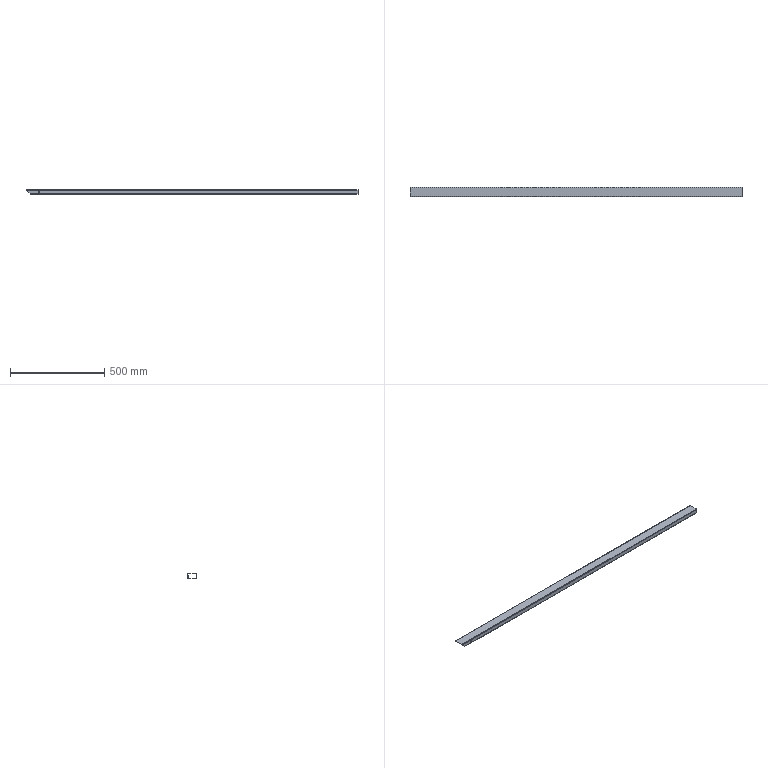Part | STEP file | Q7C0501L | 1 solid | 51 faces | box 1765 x 50 x 25 mm | volume 371060 mm3 | cylinder 23 | plane 18 | torus 10 | commonest cylinder face diameters 6 x7 9 x5 2 x4 5 x4 4 x1 8.11 x1